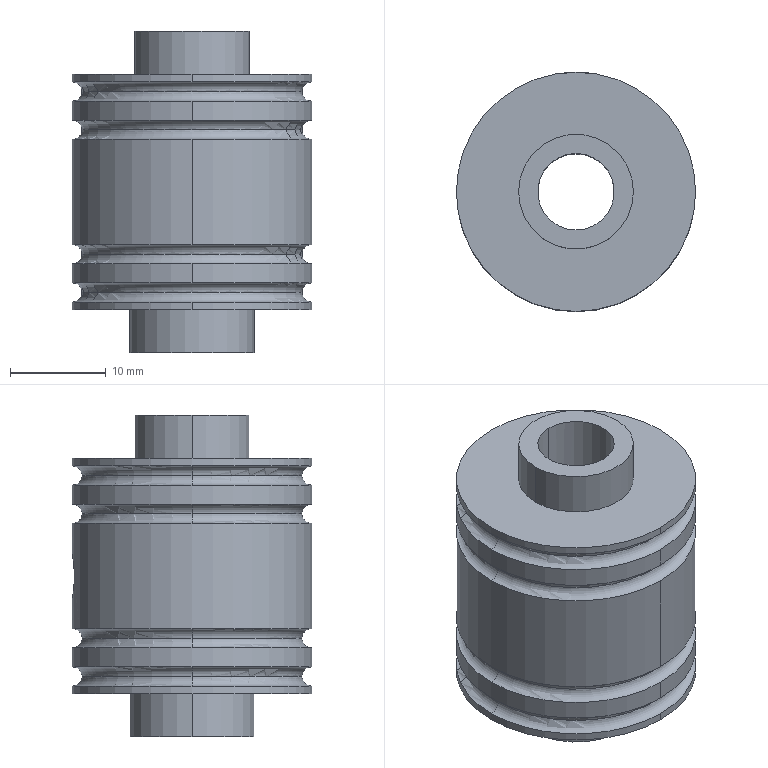Part | NX | 1 solid | 40 faces | box 25 x 25 x 33.6 mm | volume 10942 mm3 | cylinder 18 | torus 16 | plane 4 | spline 2 | commonest cylinder face diameters 25 x10 3.3 x2 8 x2 12 x2 13 x2